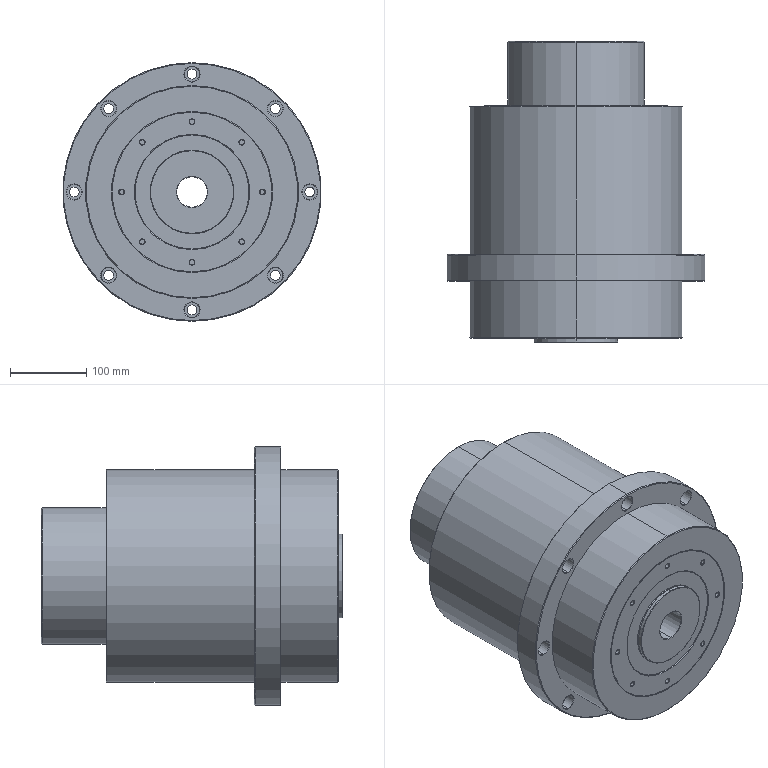Part | SolidWorks | features BaseBody 1, ICE 1 | 1 solid | 162 faces | box 340 x 396 x 340 mm | volume 21441939 mm3 | cone 66 | cylinder 64 | plane 30 | spline 2 | commonest cylinder face diameters 6.5 x16 13 x16 20 x16 280 x4 40 x2 110 x2